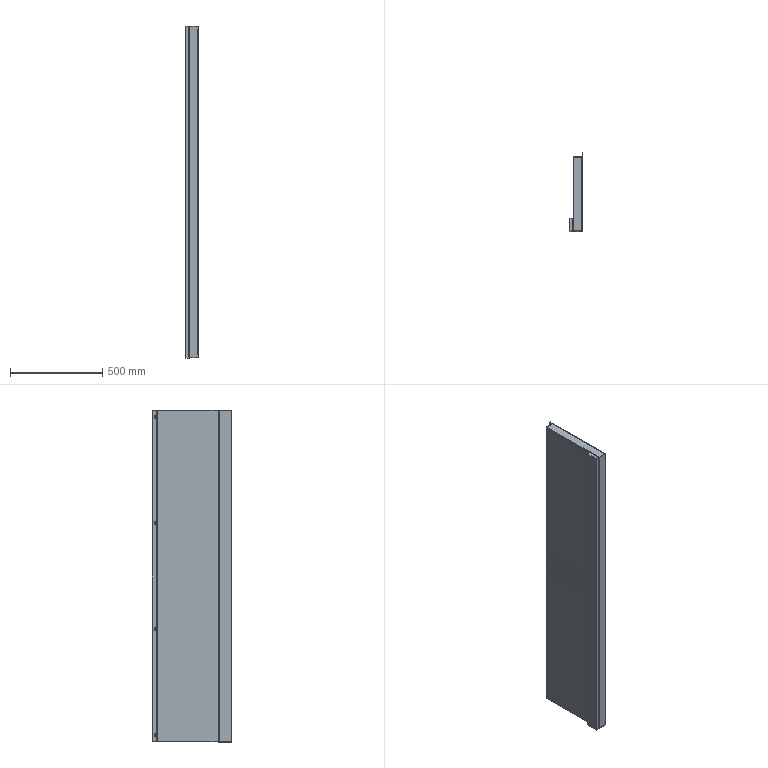Part | SolidWorks | 4 solids | 332 faces | box 70 x 430 x 1800 mm | volume 2368428 mm3 | plane 214 | cylinder 114 | spline 4 | commonest cylinder face diameters 7 x22 2 x16 6 x16 6.4 x16 5 x13 8 x11